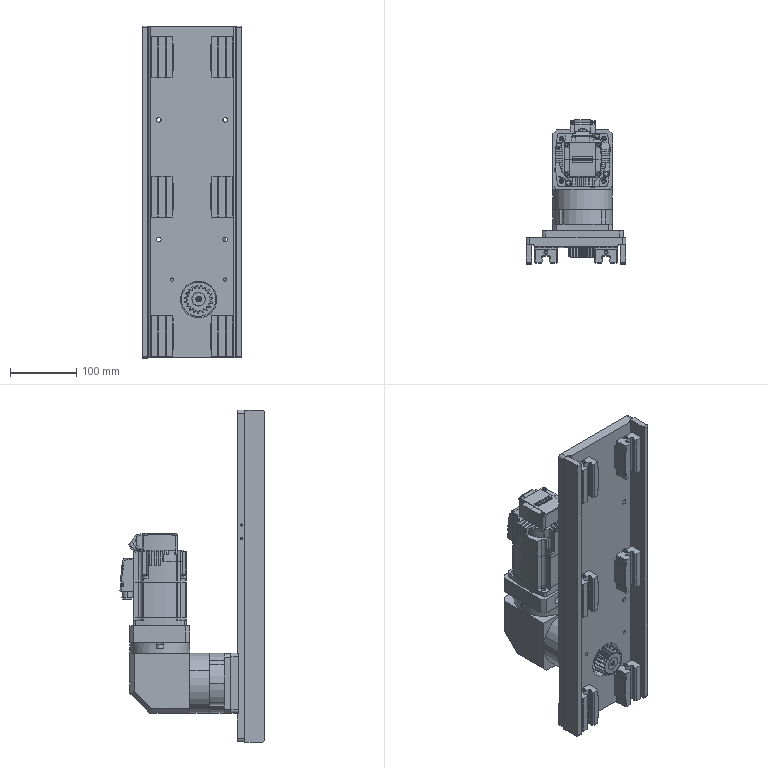Part | SolidWorks | features ReferencePattern 5, LocalLPattern 1 | 27 solids | 2677 faces | box 150 x 216.98 x 500 mm | volume 3576400 mm3 | plane 1245 | cylinder 1090 | torus 142 | sphere 118 | cone 82 | commonest cylinder face diameters 1 x116 4 x78 3.3 x76 0.8 x48 4.5 x48 5 x48